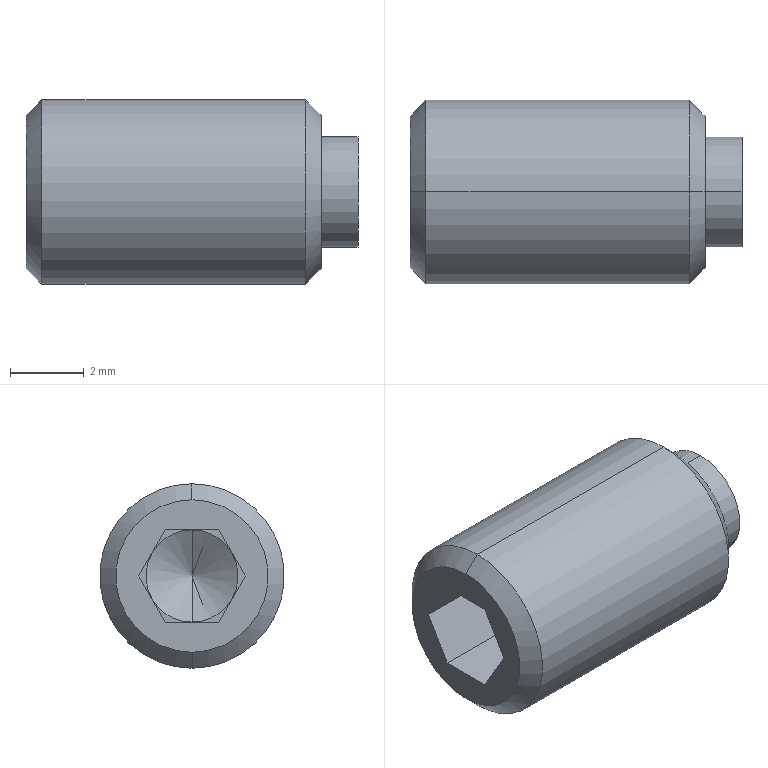Part | STEP file | 0245_007_SBPPS5-8 | 1 solid | 25 faces | box 9 x 5 x 5 mm | volume 143.954 mm3 | plane 15 | cone 6 | cylinder 4 | commonest cylinder face diameters 3 x2 5 x2